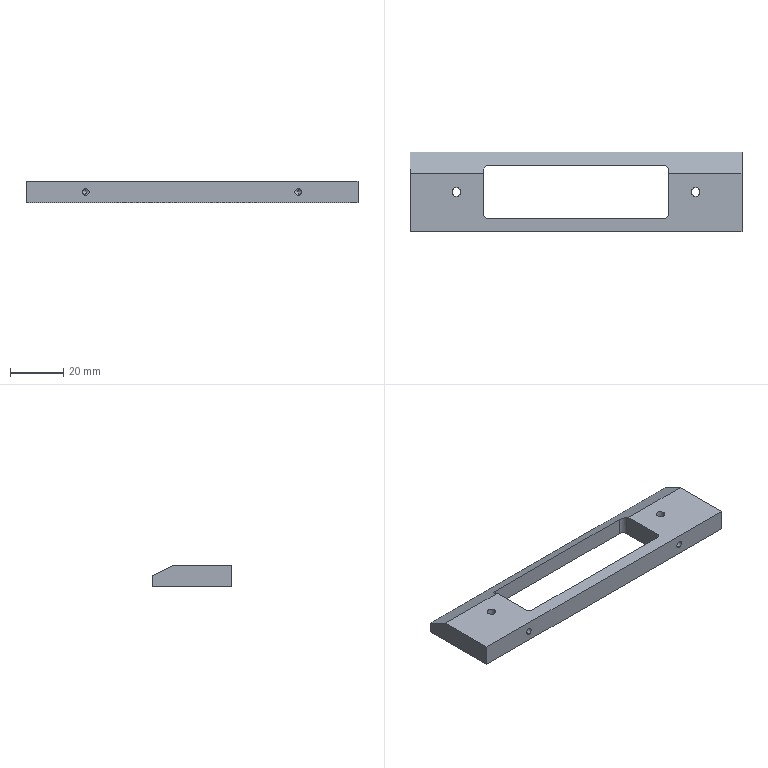Part | STEP file | XL-004 | 1 solid | 27 faces | box 125 x 30 x 8 mm | volume 16770 mm3 | cylinder 12 | plane 11 | cone 4 | commonest cylinder face diameters 2.5 x4 3.3 x4 4 x4
STEP:
#1=CARTESIAN_POINT('',(22.5,7.5,5.25));
#2=VERTEX_POINT('',#1);
#3=CARTESIAN_POINT('',(22.5,7.5,2.75));
#4=VERTEX_POINT('',#3);
#5=CARTESIAN_POINT('',(22.5,7.5,4.));
#6=DIRECTION('',(0.,-1.,0.));
#7=DIRECTION('',(0.,0.,-1.));
#8=AXIS2_PLACEMENT_3D('',#5,#6,#7);
#9=CIRCLE('',#8,1.25);
#10=EDGE_CURVE('',#2,#4,#9,.T.);
#11=ORIENTED_EDGE('',*,*,#10,.F.);
#12=CARTESIAN_POINT('',(22.5,0.,5.25));
#13=VERTEX_POINT('',#12);
#14=CARTESIAN_POINT('',(22.5,0.,5.25));
#15=DIRECTION('',(0.,-1.,0.));
#16=VECTOR('',#15,1000.);
#17=LINE('',#14,#16);
#18=EDGE_CURVE('',#2,#13,#17,.T.);
#19=ORIENTED_EDGE('',*,*,#18,.T.);
#20=CARTESIAN_POINT('',(22.5,0.,2.75));
#21=VERTEX_POINT('',#20);
#22=CARTESIAN_POINT('',(22.5,0.,4.));
#23=DIRECTION('',(0.,-1.,0.));
#24=DIRECTION('',(0.,0.,-1.));
#25=AXIS2_PLACEMENT_3D('',#22,#23,#24);
#26=CIRCLE('',#25,1.25);
#27=EDGE_CURVE('',#13,#21,#26,.T.);
#28=ORIENTED_EDGE('',*,*,#27,.T.);
#29=CARTESIAN_POINT('',(22.5,0.,2.75));
#30=DIRECTION('',(0.,-1.,0.));
#31=VECTOR('',#30,1000.);
#32=LINE('',#29,#31);
#33=EDGE_CURVE('',#4,#21,#32,.T.);
#34=ORIENTED_EDGE('',*,*,#33,.F.);
#35=EDGE_LOOP('',(#11,#19,#28,#34));
#36=FACE_OUTER_BOUND('',#35,.T.);
#37=CARTESIAN_POINT('',(22.5,0.,4.));
#38=DIRECTION('',(0.,-1.,0.));
#39=DIRECTION('',(0.,0.,-1.));
#40=AXIS2_PLACEMENT_3D('',#37,#38,#39);
#41=CYLINDRICAL_SURFACE('',#40,1.25);
#42=ADVANCED_FACE('',(#36),#41,.F.);
#43=CARTESIAN_POINT('',(22.5,8.251,4.));
#44=VERTEX_POINT('',#43);
#45=CARTESIAN_POINT('',(22.5,7.5,2.75));
#46=DIRECTION('',(0.,-0.515,-0.8572));
#47=VECTOR('',#46,1000.);
#48=LINE('',#45,#47);
#49=EDGE_CURVE('',#44,#4,#48,.T.);
#50=ORIENTED_EDGE('',*,*,#49,.F.);
#51=CARTESIAN_POINT('',(22.5,7.5,5.25));
#52=DIRECTION('',(0.,-0.515,0.8572));
#53=VECTOR('',#52,1000.);
#54=LINE('',#51,#53);
#55=EDGE_CURVE('',#44,#2,#54,.T.);
#56=ORIENTED_EDGE('',*,*,#55,.T.);
#57=ORIENTED_EDGE('',*,*,#10,.T.);
#58=EDGE_LOOP('',(#50,#56,#57));
#59=FACE_OUTER_BOUND('',#58,.T.);
#60=CARTESIAN_POINT('',(22.5,7.5,4.));
#61=DIRECTION('',(0.,-1.,0.));
#62=DIRECTION('',(0.,0.,-1.));
#63=AXIS2_PLACEMENT_3D('',#60,#61,#62);
#64=CONICAL_SURFACE('',#63,1.25,1.03);
#65=ADVANCED_FACE('',(#59),#64,.F.);
#66=CARTESIAN_POINT('',(102.5,7.5,5.25));
#67=VERTEX_POINT('',#66);
#68=CARTESIAN_POINT('',(102.5,7.5,2.75));
#69=VERTEX_POINT('',#68);
#70=CARTESIAN_POINT('',(102.5,7.5,4.));
#71=DIRECTION('',(0.,-1.,0.));
#72=DIRECTION('',(0.,0.,-1.));
#73=AXIS2_PLACEMENT_3D('',#70,#71,#72);
#74=CIRCLE('',#73,1.25);
#75=EDGE_CURVE('',#67,#69,#74,.T.);
#76=ORIENTED_EDGE('',*,*,#75,.F.);
#77=CARTESIAN_POINT('',(102.5,0.,5.25));
#78=VERTEX_POINT('',#77);
#79=CARTESIAN_POINT('',(102.5,0.,5.25));
#80=DIRECTION('',(0.,-1.,0.));
#81=VECTOR('',#80,1000.);
#82=LINE('',#79,#81);
#83=EDGE_CURVE('',#67,#78,#82,.T.);
#84=ORIENTED_EDGE('',*,*,#83,.T.);
#85=CARTESIAN_POINT('',(102.5,0.,2.75));
#86=VERTEX_POINT('',#85);
#87=CARTESIAN_POINT('',(102.5,0.,4.));
#88=DIRECTION('',(0.,-1.,0.));
#89=DIRECTION('',(0.,0.,-1.));
#90=AXIS2_PLACEMENT_3D('',#87,#88,#89);
#91=CIRCLE('',#90,1.25);
#92=EDGE_CURVE('',#78,#86,#91,.T.);
#93=ORIENTED_EDGE('',*,*,#92,.T.);
#94=CARTESIAN_POINT('',(102.5,0.,2.75));
#95=DIRECTION('',(0.,-1.,0.));
#96=VECTOR('',#95,1000.);
#97=LINE('',#94,#96);
#98=EDGE_CURVE('',#69,#86,#97,.T.);
#99=ORIENTED_EDGE('',*,*,#98,.F.);
#100=EDGE_LOOP('',(#76,#84,#93,#99));
#101=FACE_OUTER_BOUND('',#100,.T.);
#102=CARTESIAN_POINT('',(102.5,0.,4.));
#103=DIRECTION('',(0.,-1.,0.));
#104=DIRECTION('',(0.,0.,-1.));
#105=AXIS2_PLACEMENT_3D('',#102,#103,#104);
#106=CYLINDRICAL_SURFACE('',#105,1.25);
#107=ADVANCED_FACE('',(#101),#106,.F.);
#108=CARTESIAN_POINT('',(102.5,8.251,4.));
#109=VERTEX_POINT('',#108);
#110=CARTESIAN_POINT('',(102.5,7.5,2.75));
#111=DIRECTION('',(0.,-0.515,-0.8572));
#112=VECTOR('',#111,1000.);
#113=LINE('',#110,#112);
#114=EDGE_CURVE('',#109,#69,#113,.T.);
#115=ORIENTED_EDGE('',*,*,#114,.F.);
#116=CARTESIAN_POINT('',(102.5,7.5,5.25));
#117=DIRECTION('',(0.,-0.515,0.8572));
#118=VECTOR('',#117,1000.);
#119=LINE('',#116,#118);
#120=EDGE_CURVE('',#109,#67,#119,.T.);
#121=ORIENTED_EDGE('',*,*,#120,.T.);
#122=ORIENTED_EDGE('',*,*,#75,.T.);
#123=EDGE_LOOP('',(#115,#121,#122));
#124=FACE_OUTER_BOUND('',#123,.T.);
#125=CARTESIAN_POINT('',(102.5,7.5,4.));
#126=DIRECTION('',(0.,-1.,0.));
#127=DIRECTION('',(0.,0.,-1.));
#128=AXIS2_PLACEMENT_3D('',#125,#126,#127);
#129=CONICAL_SURFACE('',#128,1.25,1.03);
#130=ADVANCED_FACE('',(#124),#129,.F.);
#131=CARTESIAN_POINT('',(109.15,15.,8.));
#132=VERTEX_POINT('',#131);
#133=CARTESIAN_POINT('',(105.85,15.,8.));
#134=VERTEX_POINT('',#133);
#135=CARTESIAN_POINT('',(107.5,15.,8.));
#136=DIRECTION('',(0.,0.,-1.));
#137=DIRECTION('',(-1.,0.,0.));
#138=AXIS2_PLACEMENT_3D('',#135,#136,#137);
#139=CIRCLE('',#138,1.65);
#140=EDGE_CURVE('',#132,#134,#139,.T.);
#141=ORIENTED_EDGE('',*,*,#140,.F.);
#142=CARTESIAN_POINT('',(109.15,15.,0.));
#143=VERTEX_POINT('',#142);
#144=CARTESIAN_POINT('',(109.15,15.,0.));
#145=DIRECTION('',(0.,0.,-1.));
#146=VECTOR('',#145,1000.);
#147=LINE('',#144,#146);
#148=EDGE_CURVE('',#132,#143,#147,.T.);
#149=ORIENTED_EDGE('',*,*,#148,.T.);
#150=CARTESIAN_POINT('',(105.85,15.,0.));
#151=VERTEX_POINT('',#150);
#152=CARTESIAN_POINT('',(107.5,15.,0.));
#153=DIRECTION('',(0.,0.,-1.));
#154=DIRECTION('',(-1.,0.,0.));
#155=AXIS2_PLACEMENT_3D('',#152,#153,#154);
#156=CIRCLE('',#155,1.65);
#157=EDGE_CURVE('',#143,#151,#156,.T.);
#158=ORIENTED_EDGE('',*,*,#157,.T.);
#159=CARTESIAN_POINT('',(105.85,15.,0.));
#160=DIRECTION('',(0.,0.,-1.));
#161=VECTOR('',#160,1000.);
#162=LINE('',#159,#161);
#163=EDGE_CURVE('',#134,#151,#162,.T.);
#164=ORIENTED_EDGE('',*,*,#163,.F.);
#165=EDGE_LOOP('',(#141,#149,#158,#164));
#166=FACE_OUTER_BOUND('',#165,.T.);
#167=CARTESIAN_POINT('',(107.5,15.,0.));
#168=DIRECTION('',(0.,0.,-1.));
#169=DIRECTION('',(-1.,0.,0.));
#170=AXIS2_PLACEMENT_3D('',#167,#168,#169);
#171=CYLINDRICAL_SURFACE('',#170,1.65);
#172=ADVANCED_FACE('',(#166),#171,.F.);
#173=CARTESIAN_POINT('',(19.15,15.,8.));
#174=VERTEX_POINT('',#173);
#175=CARTESIAN_POINT('',(15.85,15.,8.));
#176=VERTEX_POINT('',#175);
#177=CARTESIAN_POINT('',(17.5,15.,8.));
#178=DIRECTION('',(0.,0.,-1.));
#179=DIRECTION('',(-1.,0.,0.));
#180=AXIS2_PLACEMENT_3D('',#177,#178,#179);
#181=CIRCLE('',#180,1.65);
#182=EDGE_CURVE('',#174,#176,#181,.T.);
#183=ORIENTED_EDGE('',*,*,#182,.F.);
#184=CARTESIAN_POINT('',(19.15,15.,0.));
#185=VERTEX_POINT('',#184);
#186=CARTESIAN_POINT('',(19.15,15.,0.));
#187=DIRECTION('',(0.,0.,-1.));
#188=VECTOR('',#187,1000.);
#189=LINE('',#186,#188);
#190=EDGE_CURVE('',#174,#185,#189,.T.);
#191=ORIENTED_EDGE('',*,*,#190,.T.);
#192=CARTESIAN_POINT('',(15.85,15.,0.));
#193=VERTEX_POINT('',#192);
#194=CARTESIAN_POINT('',(17.5,15.,0.));
#195=DIRECTION('',(0.,0.,-1.));
#196=DIRECTION('',(-1.,0.,0.));
#197=AXIS2_PLACEMENT_3D('',#194,#195,#196);
#198=CIRCLE('',#197,1.65);
#199=EDGE_CURVE('',#185,#193,#198,.T.);
#200=ORIENTED_EDGE('',*,*,#199,.T.);
#201=CARTESIAN_POINT('',(15.85,15.,0.));
#202=DIRECTION('',(0.,0.,-1.));
#203=VECTOR('',#202,1000.);
#204=LINE('',#201,#203);
#205=EDGE_CURVE('',#176,#193,#204,.T.);
#206=ORIENTED_EDGE('',*,*,#205,.F.);
#207=EDGE_LOOP('',(#183,#191,#200,#206));
#208=FACE_OUTER_BOUND('',#207,.T.);
#209=CARTESIAN_POINT('',(17.5,15.,0.));
#210=DIRECTION('',(0.,0.,-1.));
#211=DIRECTION('',(-1.,0.,0.));
#212=AXIS2_PLACEMENT_3D('',#209,#210,#211);
#213=CYLINDRICAL_SURFACE('',#212,1.65);
#214=ADVANCED_FACE('',(#208),#213,.F.);
#215=CARTESIAN_POINT('',(0.,22.,8.));
#216=VERTEX_POINT('',#215);
#217=CARTESIAN_POINT('',(0.,0.,8.));
#218=VERTEX_POINT('',#217);
#219=CARTESIAN_POINT('',(0.,0.,8.));
#220=DIRECTION('',(0.,-1.,0.));
#221=VECTOR('',#220,1000.);
#222=LINE('',#219,#221);
#223=EDGE_CURVE('',#216,#218,#222,.T.);
#224=ORIENTED_EDGE('',*,*,#223,.F.);
#225=CARTESIAN_POINT('',(0.,30.,4.));
#226=VERTEX_POINT('',#225);
#227=CARTESIAN_POINT('',(0.,30.,4.));
#228=DIRECTION('',(0.,0.8944,-0.4472));
#229=VECTOR('',#228,1000.);
#230=LINE('',#227,#229);
#231=EDGE_CURVE('',#216,#226,#230,.T.);
#232=ORIENTED_EDGE('',*,*,#231,.T.);
#233=CARTESIAN_POINT('',(0.,30.,0.));
#234=VERTEX_POINT('',#233);
#235=CARTESIAN_POINT('',(0.,30.,8.));
#236=DIRECTION('',(0.,0.,-1.));
#237=VECTOR('',#236,1000.);
#238=LINE('',#235,#237);
#239=EDGE_CURVE('',#226,#234,#238,.T.);
#240=ORIENTED_EDGE('',*,*,#239,.T.);
#241=CARTESIAN_POINT('',(0.,0.,0.));
#242=VERTEX_POINT('',#241);
#243=CARTESIAN_POINT('',(0.,0.,0.));
#244=DIRECTION('',(0.,-1.,0.));
#245=VECTOR('',#244,1000.);
#246=LINE('',#243,#245);
#247=EDGE_CURVE('',#234,#242,#246,.T.);
#248=ORIENTED_EDGE('',*,*,#247,.T.);
#249=CARTESIAN_POINT('',(0.,0.,8.));
#250=DIRECTION('',(0.,0.,-1.));
#251=VECTOR('',#250,1000.);
#252=LINE('',#249,#251);
#253=EDGE_CURVE('',#218,#242,#252,.T.);
#254=ORIENTED_EDGE('',*,*,#253,.F.);
#255=EDGE_LOOP('',(#224,#232,#240,#248,#254));
#256=FACE_OUTER_BOUND('',#255,.T.);
#257=CARTESIAN_POINT('',(0.,0.,8.));
#258=DIRECTION('',(1.,0.,0.));
#259=DIRECTION('',(0.,0.,-1.));
#260=AXIS2_PLACEMENT_3D('',#257,#258,#259);
#261=PLANE('',#260);
#262=ADVANCED_FACE('',(#256),#261,.F.);
#263=CARTESIAN_POINT('',(22.5,0.,4.));
#264=DIRECTION('',(0.,-1.,0.));
#265=DIRECTION('',(0.,0.,-1.));
#266=AXIS2_PLACEMENT_3D('',#263,#264,#265);
#267=CIRCLE('',#266,1.25);
#268=EDGE_CURVE('',#21,#13,#267,.T.);
#269=ORIENTED_EDGE('',*,*,#268,.F.);
#270=ORIENTED_EDGE('',*,*,#27,.F.);
#271=EDGE_LOOP('',(#269,#270));
#272=FACE_BOUND('',#271,.T.);
#273=CARTESIAN_POINT('',(102.5,0.,4.));
#274=DIRECTION('',(0.,-1.,0.));
#275=DIRECTION('',(0.,0.,-1.));
#276=AXIS2_PLACEMENT_3D('',#273,#274,#275);
#277=CIRCLE('',#276,1.25);
#278=EDGE_CURVE('',#86,#78,#277,.T.);
#279=ORIENTED_EDGE('',*,*,#278,.F.);
#280=ORIENTED_EDGE('',*,*,#92,.F.);
#281=EDGE_LOOP('',(#279,#280));
#282=FACE_BOUND('',#281,.T.);
#283=CARTESIAN_POINT('',(125.,0.,0.));
#284=VERTEX_POINT('',#283);
#285=CARTESIAN_POINT('',(0.,0.,0.));
#286=DIRECTION('',(1.,0.,0.));
#287=VECTOR('',#286,1000.);
#288=LINE('',#285,#287);
#289=EDGE_CURVE('',#242,#284,#288,.T.);
#290=ORIENTED_EDGE('',*,*,#289,.T.);
#291=CARTESIAN_POINT('',(125.,0.,8.));
#292=VERTEX_POINT('',#291);
#293=CARTESIAN_POINT('',(125.,0.,8.));
#294=DIRECTION('',(0.,0.,-1.));
#295=VECTOR('',#294,1000.);
#296=LINE('',#293,#295);
#297=EDGE_CURVE('',#292,#284,#296,.T.);
#298=ORIENTED_EDGE('',*,*,#297,.F.);
#299=CARTESIAN_POINT('',(0.,0.,8.));
#300=DIRECTION('',(1.,0.,0.));
#301=VECTOR('',#300,1000.);
#302=LINE('',#299,#301);
#303=EDGE_CURVE('',#218,#292,#302,.T.);
#304=ORIENTED_EDGE('',*,*,#303,.F.);
#305=ORIENTED_EDGE('',*,*,#253,.T.);
#306=EDGE_LOOP('',(#290,#298,#304,#305));
#307=FACE_OUTER_BOUND('',#306,.T.);
#308=CARTESIAN_POINT('',(0.,0.,8.));
#309=DIRECTION('',(0.,1.,0.));
#310=DIRECTION('',(0.,0.,1.));
#311=AXIS2_PLACEMENT_3D('',#308,#309,#310);
#312=PLANE('',#311);
#313=ADVANCED_FACE('',(#272,#282,#307),#312,.F.);
#314=CARTESIAN_POINT('',(125.,30.,4.));
#315=VERTEX_POINT('',#314);
#316=CARTESIAN_POINT('',(125.,30.,0.));
#317=VERTEX_POINT('',#316);
#318=CARTESIAN_POINT('',(125.,30.,8.));
#319=DIRECTION('',(0.,0.,-1.));
#320=VECTOR('',#319,1000.);
#321=LINE('',#318,#320);
#322=EDGE_CURVE('',#315,#317,#321,.T.);
#323=ORIENTED_EDGE('',*,*,#322,.F.);
#324=CARTESIAN_POINT('',(125.,22.,8.));
#325=VERTEX_POINT('',#324);
#326=CARTESIAN_POINT('',(125.,30.,4.));
#327=DIRECTION('',(0.,0.8944,-0.4472));
#328=VECTOR('',#327,1000.);
#329=LINE('',#326,#328);
#330=EDGE_CURVE('',#325,#315,#329,.T.);
#331=ORIENTED_EDGE('',*,*,#330,.F.);
#332=CARTESIAN_POINT('',(125.,0.,8.));
#333=DIRECTION('',(0.,1.,0.));
#334=VECTOR('',#333,1000.);
#335=LINE('',#332,#334);
#336=EDGE_CURVE('',#292,#325,#335,.T.);
#337=ORIENTED_EDGE('',*,*,#336,.F.);
#338=ORIENTED_EDGE('',*,*,#297,.T.);
#339=CARTESIAN_POINT('',(125.,0.,0.));
#340=DIRECTION('',(0.,1.,0.));
#341=VECTOR('',#340,1000.);
#342=LINE('',#339,#341);
#343=EDGE_CURVE('',#284,#317,#342,.T.);
#344=ORIENTED_EDGE('',*,*,#343,.T.);
#345=EDGE_LOOP('',(#323,#331,#337,#338,#344));
#346=FACE_OUTER_BOUND('',#345,.T.);
#347=CARTESIAN_POINT('',(125.,0.,8.));
#348=DIRECTION('',(-1.,0.,0.));
#349=DIRECTION('',(0.,0.,1.));
#350=AXIS2_PLACEMENT_3D('',#347,#348,#349);
#351=PLANE('',#350);
#352=ADVANCED_FACE('',(#346),#351,.F.);
#353=ORIENTED_EDGE('',*,*,#239,.F.);
#354=CARTESIAN_POINT('',(0.,30.,4.));
#355=DIRECTION('',(1.,0.,0.));
#356=VECTOR('',#355,1000.);
#357=LINE('',#354,#356);
#358=EDGE_CURVE('',#226,#315,#357,.T.);
#359=ORIENTED_EDGE('',*,*,#358,.T.);
#360=ORIENTED_EDGE('',*,*,#322,.T.);
#361=CARTESIAN_POINT('',(0.,30.,0.));
#362=DIRECTION('',(-1.,0.,0.));
#363=VECTOR('',#362,1000.);
#364=LINE('',#361,#363);
#365=EDGE_CURVE('',#317,#234,#364,.T.);
#366=ORIENTED_EDGE('',*,*,#365,.T.);
#367=EDGE_LOOP('',(#353,#359,#360,#366));
#368=FACE_OUTER_BOUND('',#367,.T.);
#369=CARTESIAN_POINT('',(0.,30.,8.));
#370=DIRECTION('',(0.,-1.,0.));
#371=DIRECTION('',(0.,0.,-1.));
#372=AXIS2_PLACEMENT_3D('',#369,#370,#371);
#373=PLANE('',#372);
#374=ADVANCED_FACE('',(#368),#373,.F.);
#375=CARTESIAN_POINT('',(107.5,15.,8.));
#376=DIRECTION('',(0.,0.,-1.));
#377=DIRECTION('',(-1.,0.,0.));
#378=AXIS2_PLACEMENT_3D('',#375,#376,#377);
#379=CIRCLE('',#378,1.65);
#380=EDGE_CURVE('',#134,#132,#379,.T.);
#381=ORIENTED_EDGE('',*,*,#380,.T.);
#382=ORIENTED_EDGE('',*,*,#140,.T.);
#383=EDGE_LOOP('',(#381,#382));
#384=FACE_BOUND('',#383,.T.);
#385=CARTESIAN_POINT('',(17.5,15.,8.));
#386=DIRECTION('',(0.,0.,-1.));
#387=DIRECTION('',(-1.,0.,0.));
#388=AXIS2_PLACEMENT_3D('',#385,#386,#387);
#389=CIRCLE('',#388,1.65);
#390=EDGE_CURVE('',#176,#174,#389,.T.);
#391=ORIENTED_EDGE('',*,*,#390,.T.);
#392=ORIENTED_EDGE('',*,*,#182,.T.);
#393=EDGE_LOOP('',(#391,#392));
#394=FACE_BOUND('',#393,.T.);
#395=CARTESIAN_POINT('',(29.5,5.,8.));
#396=VERTEX_POINT('',#395);
#397=CARTESIAN_POINT('',(27.5,7.,8.));
#398=VERTEX_POINT('',#397);
#399=CARTESIAN_POINT('',(29.5,7.,8.));
#400=DIRECTION('',(0.,0.,-1.));
#401=DIRECTION('',(-1.,0.,0.));
#402=AXIS2_PLACEMENT_3D('',#399,#400,#401);
#403=CIRCLE('',#402,2.);
#404=EDGE_CURVE('',#396,#398,#403,.T.);
#405=ORIENTED_EDGE('',*,*,#404,.T.);
#406=CARTESIAN_POINT('',(27.5,22.,8.));
#407=VERTEX_POINT('',#406);
#408=CARTESIAN_POINT('',(27.5,7.,8.));
#409=DIRECTION('',(0.,1.,0.));
#410=VECTOR('',#409,1000.);
#411=LINE('',#408,#410);
#412=EDGE_CURVE('',#398,#407,#411,.T.);
#413=ORIENTED_EDGE('',*,*,#412,.T.);
#414=CARTESIAN_POINT('',(0.,22.,8.));
#415=DIRECTION('',(1.,0.,0.));
#416=VECTOR('',#415,1000.);
#417=LINE('',#414,#416);
#418=EDGE_CURVE('',#216,#407,#417,.T.);
#419=ORIENTED_EDGE('',*,*,#418,.F.);
#420=ORIENTED_EDGE('',*,*,#223,.T.);
#421=ORIENTED_EDGE('',*,*,#303,.T.);
#422=ORIENTED_EDGE('',*,*,#336,.T.);
#423=CARTESIAN_POINT('',(97.5,22.,8.));
#424=VERTEX_POINT('',#423);
#425=CARTESIAN_POINT('',(0.,22.,8.));
#426=DIRECTION('',(1.,0.,0.));
#427=VECTOR('',#426,1000.);
#428=LINE('',#425,#427);
#429=EDGE_CURVE('',#424,#325,#428,.T.);
#430=ORIENTED_EDGE('',*,*,#429,.F.);
#431=CARTESIAN_POINT('',(97.5,7.,8.));
#432=VERTEX_POINT('',#431);
#433=CARTESIAN_POINT('',(97.5,7.,8.));
#434=DIRECTION('',(0.,-1.,0.));
#435=VECTOR('',#434,1000.);
#436=LINE('',#433,#435);
#437=EDGE_CURVE('',#424,#432,#436,.T.);
#438=ORIENTED_EDGE('',*,*,#437,.T.);
#439=CARTESIAN_POINT('',(95.5,5.,8.));
#440=VERTEX_POINT('',#439);
#441=CARTESIAN_POINT('',(95.5,7.,8.));
#442=DIRECTION('',(0.,0.,-1.));
#443=DIRECTION('',(1.,0.,0.));
#444=AXIS2_PLACEMENT_3D('',#441,#442,#443);
#445=CIRCLE('',#444,2.);
#446=EDGE_CURVE('',#432,#440,#445,.T.);
#447=ORIENTED_EDGE('',*,*,#446,.T.);
#448=CARTESIAN_POINT('',(95.5,5.,8.));
#449=DIRECTION('',(-1.,0.,0.));
#450=VECTOR('',#449,1000.);
#451=LINE('',#448,#450);
#452=EDGE_CURVE('',#440,#396,#451,.T.);
#453=ORIENTED_EDGE('',*,*,#452,.T.);
#454=EDGE_LOOP('',(#405,#413,#419,#420,#421,#422,#430,#438,#447,#453));
#455=FACE_OUTER_BOUND('',#454,.T.);
#456=CARTESIAN_POINT('',(0.,0.,8.));
#457=DIRECTION('',(0.,0.,-1.));
#458=DIRECTION('',(-1.,0.,0.));
#459=AXIS2_PLACEMENT_3D('',#456,#457,#458);
#460=PLANE('',#459);
#461=ADVANCED_FACE('',(#384,#394,#455),#460,.F.);
#462=CARTESIAN_POINT('',(107.5,15.,0.));
#463=DIRECTION('',(0.,0.,-1.));
#464=DIRECTION('',(-1.,0.,0.));
#465=AXIS2_PLACEMENT_3D('',#462,#463,#464);
#466=CIRCLE('',#465,1.65);
#467=EDGE_CURVE('',#151,#143,#466,.T.);
#468=ORIENTED_EDGE('',*,*,#467,.F.);
#469=ORIENTED_EDGE('',*,*,#157,.F.);
#470=EDGE_LOOP('',(#468,#469));
#471=FACE_BOUND('',#470,.T.);
#472=CARTESIAN_POINT('',(17.5,15.,0.));
#473=DIRECTION('',(0.,0.,-1.));
#474=DIRECTION('',(-1.,0.,0.));
#475=AXIS2_PLACEMENT_3D('',#472,#473,#474);
#476=CIRCLE('',#475,1.65);
#477=EDGE_CURVE('',#193,#185,#476,.T.);
#478=ORIENTED_EDGE('',*,*,#477,.F.);
#479=ORIENTED_EDGE('',*,*,#199,.F.);
#480=EDGE_LOOP('',(#478,#479));
#481=FACE_BOUND('',#480,.T.);
#482=CARTESIAN_POINT('',(27.5,23.,0.));
#483=VERTEX_POINT('',#482);
#484=CARTESIAN_POINT('',(29.5,25.,0.));
#485=VERTEX_POINT('',#484);
#486=CARTESIAN_POINT('',(29.5,23.,0.));
#487=DIRECTION('',(0.,0.,-1.));
#488=DIRECTION('',(1.,0.,0.));
#489=AXIS2_PLACEMENT_3D('',#486,#487,#488);
#490=CIRCLE('',#489,2.);
#491=EDGE_CURVE('',#483,#485,#490,.T.);
#492=ORIENTED_EDGE('',*,*,#491,.F.);
#493=CARTESIAN_POINT('',(27.5,7.,0.));
#494=VERTEX_POINT('',#493);
#495=CARTESIAN_POINT('',(27.5,7.,0.));
#496=DIRECTION('',(0.,1.,0.));
#497=VECTOR('',#496,1000.);
#498=LINE('',#495,#497);
#499=EDGE_CURVE('',#494,#483,#498,.T.);
#500=ORIENTED_EDGE('',*,*,#499,.F.);
#501=CARTESIAN_POINT('',(29.5,5.,0.));
#502=VERTEX_POINT('',#501);
#503=CARTESIAN_POINT('',(29.5,7.,0.));
#504=DIRECTION('',(0.,0.,-1.));
#505=DIRECTION('',(-1.,0.,0.));
#506=AXIS2_PLACEMENT_3D('',#503,#504,#505);
#507=CIRCLE('',#506,2.);
#508=EDGE_CURVE('',#502,#494,#507,.T.);
#509=ORIENTED_EDGE('',*,*,#508,.F.);
#510=CARTESIAN_POINT('',(95.5,5.,0.));
#511=VERTEX_POINT('',#510);
#512=CARTESIAN_POINT('',(95.5,5.,0.));
#513=DIRECTION('',(-1.,0.,0.));
#514=VECTOR('',#513,1000.);
#515=LINE('',#512,#514);
#516=EDGE_CURVE('',#511,#502,#515,.T.);
#517=ORIENTED_EDGE('',*,*,#516,.F.);
#518=CARTESIAN_POINT('',(97.5,7.,0.));
#519=VERTEX_POINT('',#518);
#520=CARTESIAN_POINT('',(95.5,7.,0.));
#521=DIRECTION('',(0.,0.,-1.));
#522=DIRECTION('',(1.,0.,0.));
#523=AXIS2_PLACEMENT_3D('',#520,#521,#522);
#524=CIRCLE('',#523,2.);
#525=EDGE_CURVE('',#519,#511,#524,.T.);
#526=ORIENTED_EDGE('',*,*,#525,.F.);
#527=CARTESIAN_POINT('',(97.5,23.,0.));
#528=VERTEX_POINT('',#527);
#529=CARTESIAN_POINT('',(97.5,7.,0.));
#530=DIRECTION('',(0.,-1.,0.));
#531=VECTOR('',#530,1000.);
#532=LINE('',#529,#531);
#533=EDGE_CURVE('',#528,#519,#532,.T.);
#534=ORIENTED_EDGE('',*,*,#533,.F.);
#535=CARTESIAN_POINT('',(95.5,25.,0.));
#536=VERTEX_POINT('',#535);
#537=CARTESIAN_POINT('',(95.5,23.,0.));
#538=DIRECTION('',(0.,0.,-1.));
#539=DIRECTION('',(1.,0.,0.));
#540=AXIS2_PLACEMENT_3D('',#537,#538,#539);
#541=CIRCLE('',#540,2.);
#542=EDGE_CURVE('',#536,#528,#541,.T.);
#543=ORIENTED_EDGE('',*,*,#542,.F.);
#544=CARTESIAN_POINT('',(95.5,25.,0.));
#545=DIRECTION('',(1.,0.,0.));
#546=VECTOR('',#545,1000.);
#547=LINE('',#544,#546);
#548=EDGE_CURVE('',#485,#536,#547,.T.);
#549=ORIENTED_EDGE('',*,*,#548,.F.);
#550=EDGE_LOOP('',(#492,#500,#509,#517,#526,#534,#543,#549));
#551=FACE_BOUND('',#550,.T.);
#552=ORIENTED_EDGE('',*,*,#247,.F.);
#553=ORIENTED_EDGE('',*,*,#365,.F.);
#554=ORIENTED_EDGE('',*,*,#343,.F.);
#555=ORIENTED_EDGE('',*,*,#289,.F.);
#556=EDGE_LOOP('',(#552,#553,#554,#555));
#557=FACE_OUTER_BOUND('',#556,.T.);
#558=CARTESIAN_POINT('',(0.,0.,0.));
#559=DIRECTION('',(0.,0.,-1.));
#560=DIRECTION('',(-1.,0.,0.));
#561=AXIS2_PLACEMENT_3D('',#558,#559,#560);
#562=PLANE('',#561);
#563=ADVANCED_FACE('',(#471,#481,#551,#557),#562,.T.);
#564=ORIENTED_EDGE('',*,*,#418,.T.);
#565=CARTESIAN_POINT('',(27.5,23.,7.5));
#566=VERTEX_POINT('',#565);
#567=CARTESIAN_POINT('',(27.5,30.,4.));
#568=DIRECTION('',(0.,0.8944,-0.4472));
#569=VECTOR('',#568,1000.);
#570=LINE('',#567,#569);
#571=EDGE_CURVE('',#407,#566,#570,.T.);
#572=ORIENTED_EDGE('',*,*,#571,.T.);
#573=CARTESIAN_POINT('',(29.5,25.,6.5));
#574=VERTEX_POINT('',#573);
#575=CARTESIAN_POINT('',(27.5,23.,7.5));
#576=CARTESIAN_POINT('',(27.5,24.172,6.914));
#577=CARTESIAN_POINT('',(28.328,25.,6.5));
#578=CARTESIAN_POINT('',(29.5,25.,6.5));
#579=(BOUNDED_CURVE()B_SPLINE_CURVE(3,(#575,#576,#577,#578),.UNSPECIFIED.,.F.,.F.)B_SPLINE_CURVE_WITH_KNOTS((4,4),(4.712,6.283),.UNSPECIFIED.)CURVE()GEOMETRIC_REPRESENTATION_ITEM()RATIONAL_B_SPLINE_CURVE((1.,0.8047,0.8047,1.))REPRESENTATION_ITEM(''));
#580=EDGE_CURVE('',#566,#574,#579,.T.);
#581=ORIENTED_EDGE('',*,*,#580,.T.);
#582=CARTESIAN_POINT('',(95.5,25.,6.5));
#583=VERTEX_POINT('',#582);
#584=CARTESIAN_POINT('',(0.,25.,6.5));
#585=DIRECTION('',(1.,0.,0.));
#586=VECTOR('',#585,1000.);
#587=LINE('',#584,#586);
#588=EDGE_CURVE('',#574,#583,#587,.T.);
#589=ORIENTED_EDGE('',*,*,#588,.T.);
#590=CARTESIAN_POINT('',(97.5,23.,7.5));
#591=VERTEX_POINT('',#590);
#592=CARTESIAN_POINT('',(95.5,25.,6.5));
#593=CARTESIAN_POINT('',(96.672,25.,6.5));
#594=CARTESIAN_POINT('',(97.5,24.172,6.914));
#595=CARTESIAN_POINT('',(97.5,23.,7.5));
#596=(BOUNDED_CURVE()B_SPLINE_CURVE(3,(#592,#593,#594,#595),.UNSPECIFIED.,.F.,.F.)B_SPLINE_CURVE_WITH_KNOTS((4,4),(0.,1.571),.UNSPECIFIED.)CURVE()GEOMETRIC_REPRESENTATION_ITEM()RATIONAL_B_SPLINE_CURVE((1.,0.8047,0.8047,1.))REPRESENTATION_ITEM(''));
#597=EDGE_CURVE('',#583,#591,#596,.T.);
#598=ORIENTED_EDGE('',*,*,#597,.T.);
#599=CARTESIAN_POINT('',(97.5,30.,4.));
#600=DIRECTION('',(0.,-0.8944,0.4472));
#601=VECTOR('',#600,1000.);
#602=LINE('',#599,#601);
#603=EDGE_CURVE('',#591,#424,#602,.T.);
#604=ORIENTED_EDGE('',*,*,#603,.T.);
#605=ORIENTED_EDGE('',*,*,#429,.T.);
#606=ORIENTED_EDGE('',*,*,#330,.T.);
#607=ORIENTED_EDGE('',*,*,#358,.F.);
#608=ORIENTED_EDGE('',*,*,#231,.F.);
#609=EDGE_LOOP('',(#564,#572,#581,#589,#598,#604,#605,#606,#607,#608));
#610=FACE_OUTER_BOUND('',#609,.T.);
#611=CARTESIAN_POINT('',(0.,30.,4.));
#612=DIRECTION('',(0.,-0.4472,-0.8944));
#613=DIRECTION('',(0.,0.8944,-0.4472));
#614=AXIS2_PLACEMENT_3D('',#611,#612,#613);
#615=PLANE('',#614);
#616=ADVANCED_FACE('',(#610),#615,.F.);
#617=CARTESIAN_POINT('',(27.5,23.,8.));
#618=DIRECTION('',(0.,0.,-1.));
#619=VECTOR('',#618,1000.);
#620=LINE('',#617,#619);
#621=EDGE_CURVE('',#566,#483,#620,.T.);
#622=ORIENTED_EDGE('',*,*,#621,.T.);
#623=ORIENTED_EDGE('',*,*,#491,.T.);
#624=CARTESIAN_POINT('',(29.5,25.,8.));
#625=DIRECTION('',(0.,0.,-1.));
#626=VECTOR('',#625,1000.);
#627=LINE('',#624,#626);
#628=EDGE_CURVE('',#574,#485,#627,.T.);
#629=ORIENTED_EDGE('',*,*,#628,.F.);
#630=ORIENTED_EDGE('',*,*,#580,.F.);
#631=EDGE_LOOP('',(#622,#623,#629,#630));
#632=FACE_OUTER_BOUND('',#631,.T.);
#633=CARTESIAN_POINT('',(29.5,23.,8.));
#634=DIRECTION('',(0.,0.,-1.));
#635=DIRECTION('',(-1.,0.,0.));
#636=AXIS2_PLACEMENT_3D('',#633,#634,#635);
#637=CYLINDRICAL_SURFACE('',#636,2.);
#638=ADVANCED_FACE('',(#632),#637,.F.);
#639=ORIENTED_EDGE('',*,*,#412,.F.);
#640=CARTESIAN_POINT('',(27.5,7.,8.));
#641=DIRECTION('',(0.,0.,-1.));
#642=VECTOR('',#641,1000.);
#643=LINE('',#640,#642);
#644=EDGE_CURVE('',#398,#494,#643,.T.);
#645=ORIENTED_EDGE('',*,*,#644,.T.);
#646=ORIENTED_EDGE('',*,*,#499,.T.);
#647=ORIENTED_EDGE('',*,*,#621,.F.);
#648=ORIENTED_EDGE('',*,*,#571,.F.);
#649=EDGE_LOOP('',(#639,#645,#646,#647,#648));
#650=FACE_OUTER_BOUND('',#649,.T.);
#651=CARTESIAN_POINT('',(27.5,7.,8.));
#652=DIRECTION('',(-1.,0.,0.));
#653=DIRECTION('',(0.,0.,1.));
#654=AXIS2_PLACEMENT_3D('',#651,#652,#653);
#655=PLANE('',#654);
#656=ADVANCED_FACE('',(#650),#655,.F.);
#657=CARTESIAN_POINT('',(97.5,23.,8.));
#658=DIRECTION('',(0.,0.,-1.));
#659=VECTOR('',#658,1000.);
#660=LINE('',#657,#659);
#661=EDGE_CURVE('',#591,#528,#660,.T.);
#662=ORIENTED_EDGE('',*,*,#661,.T.);
#663=ORIENTED_EDGE('',*,*,#533,.T.);
#664=CARTESIAN_POINT('',(97.5,7.,8.));
#665=DIRECTION('',(0.,0.,-1.));
#666=VECTOR('',#665,1000.);
#667=LINE('',#664,#666);
#668=EDGE_CURVE('',#432,#519,#667,.T.);
#669=ORIENTED_EDGE('',*,*,#668,.F.);
#670=ORIENTED_EDGE('',*,*,#437,.F.);
#671=ORIENTED_EDGE('',*,*,#603,.F.);
#672=EDGE_LOOP('',(#662,#663,#669,#670,#671));
#673=FACE_OUTER_BOUND('',#672,.T.);
#674=CARTESIAN_POINT('',(97.5,7.,8.));
#675=DIRECTION('',(1.,0.,0.));
#676=DIRECTION('',(0.,0.,-1.));
#677=AXIS2_PLACEMENT_3D('',#674,#675,#676);
#678=PLANE('',#677);
#679=ADVANCED_FACE('',(#673),#678,.F.);
#680=CARTESIAN_POINT('',(95.5,25.,8.));
#681=DIRECTION('',(0.,0.,-1.));
#682=VECTOR('',#681,1000.);
#683=LINE('',#680,#682);
#684=EDGE_CURVE('',#583,#536,#683,.T.);
#685=ORIENTED_EDGE('',*,*,#684,.T.);
#686=ORIENTED_EDGE('',*,*,#542,.T.);
#687=ORIENTED_EDGE('',*,*,#661,.F.);
#688=ORIENTED_EDGE('',*,*,#597,.F.);
#689=EDGE_LOOP('',(#685,#686,#687,#688));
#690=FACE_OUTER_BOUND('',#689,.T.);
#691=CARTESIAN_POINT('',(95.5,23.,8.));
#692=DIRECTION('',(0.,0.,-1.));
#693=DIRECTION('',(-1.,0.,0.));
#694=AXIS2_PLACEMENT_3D('',#691,#692,#693);
#695=CYLINDRICAL_SURFACE('',#694,2.);
#696=ADVANCED_FACE('',(#690),#695,.F.);
#697=ORIENTED_EDGE('',*,*,#628,.T.);
#698=ORIENTED_EDGE('',*,*,#548,.T.);
#699=ORIENTED_EDGE('',*,*,#684,.F.);
#700=ORIENTED_EDGE('',*,*,#588,.F.);
#701=EDGE_LOOP('',(#697,#698,#699,#700));
#702=FACE_OUTER_BOUND('',#701,.T.);
#703=CARTESIAN_POINT('',(95.5,25.,8.));
#704=DIRECTION('',(0.,1.,0.));
#705=DIRECTION('',(0.,0.,1.));
#706=AXIS2_PLACEMENT_3D('',#703,#704,#705);
#707=PLANE('',#706);
#708=ADVANCED_FACE('',(#702),#707,.F.);
#709=ORIENTED_EDGE('',*,*,#508,.T.);
#710=ORIENTED_EDGE('',*,*,#644,.F.);
#711=ORIENTED_EDGE('',*,*,#404,.F.);
#712=CARTESIAN_POINT('',(29.5,5.,8.));
#713=DIRECTION('',(0.,0.,-1.));
#714=VECTOR('',#713,1000.);
#715=LINE('',#712,#714);
#716=EDGE_CURVE('',#396,#502,#715,.T.);
#717=ORIENTED_EDGE('',*,*,#716,.T.);
#718=EDGE_LOOP('',(#709,#710,#711,#717));
#719=FACE_OUTER_BOUND('',#718,.T.);
#720=CARTESIAN_POINT('',(29.5,7.,8.));
#721=DIRECTION('',(0.,0.,-1.));
#722=DIRECTION('',(-1.,0.,0.));
#723=AXIS2_PLACEMENT_3D('',#720,#721,#722);
#724=CYLINDRICAL_SURFACE('',#723,2.);
#725=ADVANCED_FACE('',(#719),#724,.F.);
#726=ORIENTED_EDGE('',*,*,#516,.T.);
#727=ORIENTED_EDGE('',*,*,#716,.F.);
#728=ORIENTED_EDGE('',*,*,#452,.F.);
#729=CARTESIAN_POINT('',(95.5,5.,8.));
#730=DIRECTION('',(0.,0.,-1.));
#731=VECTOR('',#730,1000.);
#732=LINE('',#729,#731);
#733=EDGE_CURVE('',#440,#511,#732,.T.);
#734=ORIENTED_EDGE('',*,*,#733,.T.);
#735=EDGE_LOOP('',(#726,#727,#728,#734));
#736=FACE_OUTER_BOUND('',#735,.T.);
#737=CARTESIAN_POINT('',(95.5,5.,8.));
#738=DIRECTION('',(0.,-1.,0.));
#739=DIRECTION('',(0.,0.,-1.));
#740=AXIS2_PLACEMENT_3D('',#737,#738,#739);
#741=PLANE('',#740);
#742=ADVANCED_FACE('',(#736),#741,.F.);
#743=ORIENTED_EDGE('',*,*,#525,.T.);
#744=ORIENTED_EDGE('',*,*,#733,.F.);
#745=ORIENTED_EDGE('',*,*,#446,.F.);
#746=ORIENTED_EDGE('',*,*,#668,.T.);
#747=EDGE_LOOP('',(#743,#744,#745,#746));
#748=FACE_OUTER_BOUND('',#747,.T.);
#749=CARTESIAN_POINT('',(95.5,7.,8.));
#750=DIRECTION('',(0.,0.,-1.));
#751=DIRECTION('',(-1.,0.,0.));
#752=AXIS2_PLACEMENT_3D('',#749,#750,#751);
#753=CYLINDRICAL_SURFACE('',#752,2.);
#754=ADVANCED_FACE('',(#748),#753,.F.);
#755=ORIENTED_EDGE('',*,*,#190,.F.);
#756=ORIENTED_EDGE('',*,*,#390,.F.);
#757=ORIENTED_EDGE('',*,*,#205,.T.);
#758=ORIENTED_EDGE('',*,*,#477,.T.);
#759=EDGE_LOOP('',(#755,#756,#757,#758));
#760=FACE_OUTER_BOUND('',#759,.T.);
#761=CARTESIAN_POINT('',(17.5,15.,0.));
#762=DIRECTION('',(0.,0.,-1.));
#763=DIRECTION('',(-1.,0.,0.));
#764=AXIS2_PLACEMENT_3D('',#761,#762,#763);
#765=CYLINDRICAL_SURFACE('',#764,1.65);
#766=ADVANCED_FACE('',(#760),#765,.F.);
#767=ORIENTED_EDGE('',*,*,#148,.F.);
#768=ORIENTED_EDGE('',*,*,#380,.F.);
#769=ORIENTED_EDGE('',*,*,#163,.T.);
#770=ORIENTED_EDGE('',*,*,#467,.T.);
#771=EDGE_LOOP('',(#767,#768,#769,#770));
#772=FACE_OUTER_BOUND('',#771,.T.);
#773=CARTESIAN_POINT('',(107.5,15.,0.));
#774=DIRECTION('',(0.,0.,-1.));
#775=DIRECTION('',(-1.,0.,0.));
#776=AXIS2_PLACEMENT_3D('',#773,#774,#775);
#777=CYLINDRICAL_SURFACE('',#776,1.65);
#778=ADVANCED_FACE('',(#772),#777,.F.);
#779=ORIENTED_EDGE('',*,*,#120,.F.);
#780=ORIENTED_EDGE('',*,*,#114,.T.);
#781=CARTESIAN_POINT('',(102.5,7.5,4.));
#782=DIRECTION('',(0.,-1.,0.));
#783=DIRECTION('',(0.,0.,-1.));
#784=AXIS2_PLACEMENT_3D('',#781,#782,#783);
#785=CIRCLE('',#784,1.25);
#786=EDGE_CURVE('',#69,#67,#785,.T.);
#787=ORIENTED_EDGE('',*,*,#786,.T.);
#788=EDGE_LOOP('',(#779,#780,#787));
#789=FACE_OUTER_BOUND('',#788,.T.);
#790=CARTESIAN_POINT('',(102.5,7.5,4.));
#791=DIRECTION('',(0.,-1.,0.));
#792=DIRECTION('',(0.,0.,-1.));
#793=AXIS2_PLACEMENT_3D('',#790,#791,#792);
#794=CONICAL_SURFACE('',#793,1.25,1.03);
#795=ADVANCED_FACE('',(#789),#794,.F.);
#796=ORIENTED_EDGE('',*,*,#83,.F.);
#797=ORIENTED_EDGE('',*,*,#786,.F.);
#798=ORIENTED_EDGE('',*,*,#98,.T.);
#799=ORIENTED_EDGE('',*,*,#278,.T.);
#800=EDGE_LOOP('',(#796,#797,#798,#799));
#801=FACE_OUTER_BOUND('',#800,.T.);
#802=CARTESIAN_POINT('',(102.5,0.,4.));
#803=DIRECTION('',(0.,-1.,0.));
#804=DIRECTION('',(0.,0.,-1.));
#805=AXIS2_PLACEMENT_3D('',#802,#803,#804);
#806=CYLINDRICAL_SURFACE('',#805,1.25);
#807=ADVANCED_FACE('',(#801),#806,.F.);
#808=ORIENTED_EDGE('',*,*,#55,.F.);
#809=ORIENTED_EDGE('',*,*,#49,.T.);
#810=CARTESIAN_POINT('',(22.5,7.5,4.));
#811=DIRECTION('',(0.,-1.,0.));
#812=DIRECTION('',(0.,0.,-1.));
#813=AXIS2_PLACEMENT_3D('',#810,#811,#812);
#814=CIRCLE('',#813,1.25);
#815=EDGE_CURVE('',#4,#2,#814,.T.);
#816=ORIENTED_EDGE('',*,*,#815,.T.);
#817=EDGE_LOOP('',(#808,#809,#816));
#818=FACE_OUTER_BOUND('',#817,.T.);
#819=CARTESIAN_POINT('',(22.5,7.5,4.));
#820=DIRECTION('',(0.,-1.,0.));
#821=DIRECTION('',(0.,0.,-1.));
#822=AXIS2_PLACEMENT_3D('',#819,#820,#821);
#823=CONICAL_SURFACE('',#822,1.25,1.03);
#824=ADVANCED_FACE('',(#818),#823,.F.);
#825=ORIENTED_EDGE('',*,*,#18,.F.);
#826=ORIENTED_EDGE('',*,*,#815,.F.);
#827=ORIENTED_EDGE('',*,*,#33,.T.);
#828=ORIENTED_EDGE('',*,*,#268,.T.);
#829=EDGE_LOOP('',(#825,#826,#827,#828));
#830=FACE_OUTER_BOUND('',#829,.T.);
#831=CARTESIAN_POINT('',(22.5,0.,4.));
#832=DIRECTION('',(0.,-1.,0.));
#833=DIRECTION('',(0.,0.,-1.));
#834=AXIS2_PLACEMENT_3D('',#831,#832,#833);
#835=CYLINDRICAL_SURFACE('',#834,1.25);
#836=ADVANCED_FACE('',(#830),#835,.F.);
#837=CLOSED_SHELL('',(#42,#65,#107,#130,#172,#214,#262,#313,#352,#374,#461,#563,#616,#638,#656,#679,#696,#708,#725,#742,#754,#766,#778,#795,#807,#824,#836));
#838=MANIFOLD_SOLID_BREP('',#837);
#839=CARTESIAN_POINT('',(0.,0.,0.));
#840=DIRECTION('',(0.,0.,1.));
#841=DIRECTION('',(1.,0.,0.));
#842=AXIS2_PLACEMENT_3D('',#839,#840,#841);
#843=(LENGTH_UNIT()NAMED_UNIT(*)SI_UNIT(.MILLI.,.METRE.));
#844=UNCERTAINTY_MEASURE_WITH_UNIT(LENGTH_MEASURE(0.00001),#843,'','');
#845=(NAMED_UNIT(*)PLANE_ANGLE_UNIT()SI_UNIT($,.RADIAN.));
#846=(NAMED_UNIT(*)SI_UNIT($,.STERADIAN.)SOLID_ANGLE_UNIT());
#847=(GEOMETRIC_REPRESENTATION_CONTEXT(3)GLOBAL_UNCERTAINTY_ASSIGNED_CONTEXT((#844))GLOBAL_UNIT_ASSIGNED_CONTEXT((#843,#845,#846))REPRESENTATION_CONTEXT('',''));
#848=ADVANCED_BREP_SHAPE_REPRESENTATION('',(#838,#842),#847);